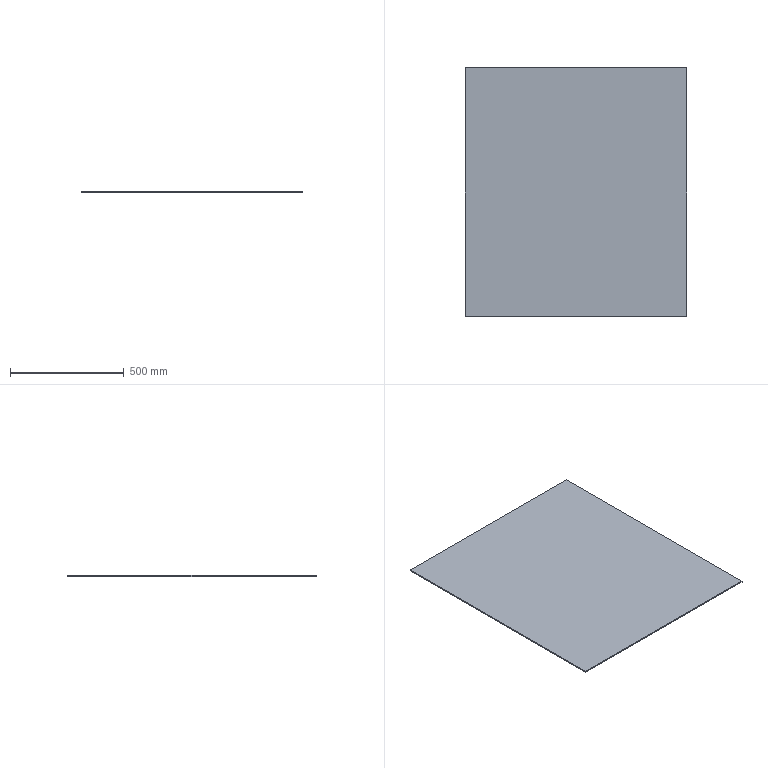Part | SolidWorks | features Extrusion 1, HoleWzd 1 | 1 solid | 6 faces | box 972 x 1092 x 5 mm | volume 5307120 mm3 | plane 6
STEP:
#1=CARTESIAN_POINT('',(486.,-546.,0.));
#2=VERTEX_POINT('',#1);
#3=CARTESIAN_POINT('',(486.,546.,0.));
#4=VERTEX_POINT('',#3);
#5=CARTESIAN_POINT('',(486.,546.,0.));
#6=DIRECTION('',(0.,1.,0.));
#7=VECTOR('',#6,1000.);
#8=LINE('',#5,#7);
#9=EDGE_CURVE('',#2,#4,#8,.T.);
#10=ORIENTED_EDGE('',*,*,#9,.T.);
#11=CARTESIAN_POINT('',(486.,546.,5.));
#12=VERTEX_POINT('',#11);
#13=CARTESIAN_POINT('',(486.,546.,5.));
#14=DIRECTION('',(0.,0.,-1.));
#15=VECTOR('',#14,1000.);
#16=LINE('',#13,#15);
#17=EDGE_CURVE('',#12,#4,#16,.T.);
#18=ORIENTED_EDGE('',*,*,#17,.F.);
#19=CARTESIAN_POINT('',(486.,-546.,5.));
#20=VERTEX_POINT('',#19);
#21=CARTESIAN_POINT('',(486.,546.,5.));
#22=DIRECTION('',(0.,1.,0.));
#23=VECTOR('',#22,1000.);
#24=LINE('',#21,#23);
#25=EDGE_CURVE('',#20,#12,#24,.T.);
#26=ORIENTED_EDGE('',*,*,#25,.F.);
#27=CARTESIAN_POINT('',(486.,-546.,5.));
#28=DIRECTION('',(0.,0.,-1.));
#29=VECTOR('',#28,1000.);
#30=LINE('',#27,#29);
#31=EDGE_CURVE('',#20,#2,#30,.T.);
#32=ORIENTED_EDGE('',*,*,#31,.T.);
#33=EDGE_LOOP('',(#10,#18,#26,#32));
#34=FACE_OUTER_BOUND('',#33,.T.);
#35=CARTESIAN_POINT('',(486.,546.,5.));
#36=DIRECTION('',(-1.,0.,0.));
#37=DIRECTION('',(0.,-1.,0.));
#38=AXIS2_PLACEMENT_3D('',#35,#36,#37);
#39=PLANE('',#38);
#40=ADVANCED_FACE('',(#34),#39,.F.);
#41=CARTESIAN_POINT('',(-486.,546.,0.));
#42=VERTEX_POINT('',#41);
#43=CARTESIAN_POINT('',(-486.,546.,0.));
#44=DIRECTION('',(-1.,0.,0.));
#45=VECTOR('',#44,1000.);
#46=LINE('',#43,#45);
#47=EDGE_CURVE('',#4,#42,#46,.T.);
#48=ORIENTED_EDGE('',*,*,#47,.T.);
#49=CARTESIAN_POINT('',(-486.,546.,5.));
#50=VERTEX_POINT('',#49);
#51=CARTESIAN_POINT('',(-486.,546.,5.));
#52=DIRECTION('',(0.,0.,-1.));
#53=VECTOR('',#52,1000.);
#54=LINE('',#51,#53);
#55=EDGE_CURVE('',#50,#42,#54,.T.);
#56=ORIENTED_EDGE('',*,*,#55,.F.);
#57=CARTESIAN_POINT('',(-486.,546.,5.));
#58=DIRECTION('',(-1.,0.,0.));
#59=VECTOR('',#58,1000.);
#60=LINE('',#57,#59);
#61=EDGE_CURVE('',#12,#50,#60,.T.);
#62=ORIENTED_EDGE('',*,*,#61,.F.);
#63=ORIENTED_EDGE('',*,*,#17,.T.);
#64=EDGE_LOOP('',(#48,#56,#62,#63));
#65=FACE_OUTER_BOUND('',#64,.T.);
#66=CARTESIAN_POINT('',(-486.,546.,5.));
#67=DIRECTION('',(0.,-1.,0.));
#68=DIRECTION('',(0.,0.,-1.));
#69=AXIS2_PLACEMENT_3D('',#66,#67,#68);
#70=PLANE('',#69);
#71=ADVANCED_FACE('',(#65),#70,.F.);
#72=CARTESIAN_POINT('',(-486.,-546.,0.));
#73=VERTEX_POINT('',#72);
#74=CARTESIAN_POINT('',(-486.,546.,0.));
#75=DIRECTION('',(0.,-1.,0.));
#76=VECTOR('',#75,1000.);
#77=LINE('',#74,#76);
#78=EDGE_CURVE('',#42,#73,#77,.T.);
#79=ORIENTED_EDGE('',*,*,#78,.T.);
#80=CARTESIAN_POINT('',(-486.,-546.,5.));
#81=VERTEX_POINT('',#80);
#82=CARTESIAN_POINT('',(-486.,-546.,5.));
#83=DIRECTION('',(0.,0.,-1.));
#84=VECTOR('',#83,1000.);
#85=LINE('',#82,#84);
#86=EDGE_CURVE('',#81,#73,#85,.T.);
#87=ORIENTED_EDGE('',*,*,#86,.F.);
#88=CARTESIAN_POINT('',(-486.,546.,5.));
#89=DIRECTION('',(0.,-1.,0.));
#90=VECTOR('',#89,1000.);
#91=LINE('',#88,#90);
#92=EDGE_CURVE('',#50,#81,#91,.T.);
#93=ORIENTED_EDGE('',*,*,#92,.F.);
#94=ORIENTED_EDGE('',*,*,#55,.T.);
#95=EDGE_LOOP('',(#79,#87,#93,#94));
#96=FACE_OUTER_BOUND('',#95,.T.);
#97=CARTESIAN_POINT('',(-486.,546.,5.));
#98=DIRECTION('',(1.,0.,0.));
#99=DIRECTION('',(0.,1.,0.));
#100=AXIS2_PLACEMENT_3D('',#97,#98,#99);
#101=PLANE('',#100);
#102=ADVANCED_FACE('',(#96),#101,.F.);
#103=CARTESIAN_POINT('',(-486.,-546.,0.));
#104=DIRECTION('',(1.,0.,0.));
#105=VECTOR('',#104,1000.);
#106=LINE('',#103,#105);
#107=EDGE_CURVE('',#73,#2,#106,.T.);
#108=ORIENTED_EDGE('',*,*,#107,.T.);
#109=ORIENTED_EDGE('',*,*,#31,.F.);
#110=CARTESIAN_POINT('',(-486.,-546.,5.));
#111=DIRECTION('',(1.,0.,0.));
#112=VECTOR('',#111,1000.);
#113=LINE('',#110,#112);
#114=EDGE_CURVE('',#81,#20,#113,.T.);
#115=ORIENTED_EDGE('',*,*,#114,.F.);
#116=ORIENTED_EDGE('',*,*,#86,.T.);
#117=EDGE_LOOP('',(#108,#109,#115,#116));
#118=FACE_OUTER_BOUND('',#117,.T.);
#119=CARTESIAN_POINT('',(-486.,-546.,5.));
#120=DIRECTION('',(0.,1.,0.));
#121=DIRECTION('',(0.,0.,1.));
#122=AXIS2_PLACEMENT_3D('',#119,#120,#121);
#123=PLANE('',#122);
#124=ADVANCED_FACE('',(#118),#123,.F.);
#125=ORIENTED_EDGE('',*,*,#25,.T.);
#126=ORIENTED_EDGE('',*,*,#61,.T.);
#127=ORIENTED_EDGE('',*,*,#92,.T.);
#128=ORIENTED_EDGE('',*,*,#114,.T.);
#129=EDGE_LOOP('',(#125,#126,#127,#128));
#130=FACE_OUTER_BOUND('',#129,.T.);
#131=CARTESIAN_POINT('',(0.,0.,5.));
#132=DIRECTION('',(0.,0.,1.));
#133=DIRECTION('',(1.,0.,0.));
#134=AXIS2_PLACEMENT_3D('',#131,#132,#133);
#135=PLANE('',#134);
#136=ADVANCED_FACE('',(#130),#135,.T.);
#137=ORIENTED_EDGE('',*,*,#9,.F.);
#138=ORIENTED_EDGE('',*,*,#107,.F.);
#139=ORIENTED_EDGE('',*,*,#78,.F.);
#140=ORIENTED_EDGE('',*,*,#47,.F.);
#141=EDGE_LOOP('',(#137,#138,#139,#140));
#142=FACE_OUTER_BOUND('',#141,.T.);
#143=CARTESIAN_POINT('',(0.,0.,0.));
#144=DIRECTION('',(0.,0.,1.));
#145=DIRECTION('',(1.,0.,0.));
#146=AXIS2_PLACEMENT_3D('',#143,#144,#145);
#147=PLANE('',#146);
#148=ADVANCED_FACE('',(#142),#147,.F.);
#149=CLOSED_SHELL('',(#40,#71,#102,#124,#136,#148));
#150=MANIFOLD_SOLID_BREP('',#149);
#151=CARTESIAN_POINT('',(0.,0.,0.));
#152=DIRECTION('',(0.,0.,1.));
#153=DIRECTION('',(1.,0.,0.));
#154=AXIS2_PLACEMENT_3D('',#151,#152,#153);
#155=(LENGTH_UNIT()NAMED_UNIT(*)SI_UNIT(.MILLI.,.METRE.));
#156=UNCERTAINTY_MEASURE_WITH_UNIT(LENGTH_MEASURE(0.00001),#155,'','');
#157=(NAMED_UNIT(*)PLANE_ANGLE_UNIT()SI_UNIT($,.RADIAN.));
#158=(NAMED_UNIT(*)SI_UNIT($,.STERADIAN.)SOLID_ANGLE_UNIT());
#159=(GEOMETRIC_REPRESENTATION_CONTEXT(3)GLOBAL_UNCERTAINTY_ASSIGNED_CONTEXT((#156))GLOBAL_UNIT_ASSIGNED_CONTEXT((#155,#157,#158))REPRESENTATION_CONTEXT('',''));
#160=ADVANCED_BREP_SHAPE_REPRESENTATION('',(#150,#154),#159);